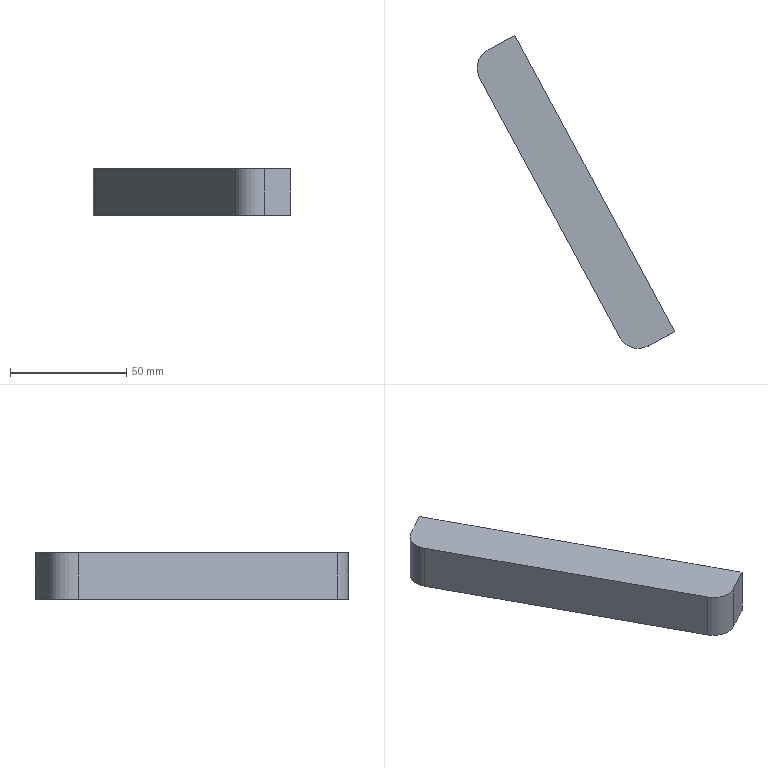Part | Creo | 1 solid | 8 faces | box 85.061 x 134.843 x 20 mm | volume 63105 mm3 | plane 6 | cylinder 2 | commonest cylinder face diameters 18 x2
STEP:
#1=CARTESIAN_POINT('',(0.,0.,0.));
#2=DIRECTION('',(0.,0.,1.));
#3=DIRECTION('',(1.,0.,0.));
#4=AXIS2_PLACEMENT_3D('',#1,#2,#3);
#5=CARTESIAN_POINT('',(223.318,-130.597,-86.844));
#6=VERTEX_POINT('',#5);
#7=CARTESIAN_POINT('',(292.216,-258.183,-86.844));
#8=VERTEX_POINT('',#7);
#9=CARTESIAN_POINT('',(223.318,-130.597,-86.844));
#10=DIRECTION('',(0.4752,-0.8799,0.));
#11=VECTOR('',#10,145.);
#12=LINE('',#9,#11);
#13=EDGE_CURVE('',#6,#8,#12,.T.);
#14=ORIENTED_EDGE('',*,*,#13,.T.);
#15=CARTESIAN_POINT('',(292.216,-258.183,-66.844));
#16=VERTEX_POINT('',#15);
#17=CARTESIAN_POINT('',(292.216,-258.183,-86.844));
#18=DIRECTION('',(0.,0.,1.));
#19=VECTOR('',#18,20.);
#20=LINE('',#17,#19);
#21=EDGE_CURVE('',#8,#16,#20,.T.);
#22=ORIENTED_EDGE('',*,*,#21,.T.);
#23=CARTESIAN_POINT('',(223.318,-130.597,-66.844));
#24=VERTEX_POINT('',#23);
#25=CARTESIAN_POINT('',(292.216,-258.183,-66.844));
#26=DIRECTION('',(-0.4752,0.8799,0.));
#27=VECTOR('',#26,145.);
#28=LINE('',#25,#27);
#29=EDGE_CURVE('',#16,#24,#28,.T.);
#30=ORIENTED_EDGE('',*,*,#29,.T.);
#31=CARTESIAN_POINT('',(223.318,-130.597,-86.844));
#32=DIRECTION('',(0.,0.,1.));
#33=VECTOR('',#32,20.);
#34=LINE('',#31,#33);
#35=EDGE_CURVE('',#6,#24,#34,.T.);
#36=ORIENTED_EDGE('',*,*,#35,.F.);
#37=EDGE_LOOP('',(#14,#22,#30,#36));
#38=FACE_OUTER_BOUND('',#37,.F.);
#39=CARTESIAN_POINT('',(270.834,-218.587,-66.844));
#40=DIRECTION('',(-0.8799,-0.4752,0.));
#41=DIRECTION('',(0.4752,-0.8799,0.));
#42=AXIS2_PLACEMENT_3D('',#39,#40,#41);
#43=PLANE('',#42);
#44=ADVANCED_FACE('',(#38),#43,.F.);
#45=CARTESIAN_POINT('',(280.778,-264.36,-86.844));
#46=VERTEX_POINT('',#45);
#47=CARTESIAN_POINT('',(292.216,-258.183,-86.844));
#48=DIRECTION('',(-0.8799,-0.4752,0.));
#49=VECTOR('',#48,13.);
#50=LINE('',#47,#49);
#51=EDGE_CURVE('',#8,#46,#50,.T.);
#52=ORIENTED_EDGE('',*,*,#51,.F.);
#53=ORIENTED_EDGE('',*,*,#13,.F.);
#54=CARTESIAN_POINT('',(211.879,-136.775,-86.844));
#55=VERTEX_POINT('',#54);
#56=CARTESIAN_POINT('',(211.879,-136.775,-86.844));
#57=DIRECTION('',(0.8799,0.4752,0.));
#58=VECTOR('',#57,13.);
#59=LINE('',#56,#58);
#60=EDGE_CURVE('',#55,#6,#59,.T.);
#61=ORIENTED_EDGE('',*,*,#60,.F.);
#62=CARTESIAN_POINT('',(208.237,-148.97,-86.844));
#63=VERTEX_POINT('',#62);
#64=CARTESIAN_POINT('',(216.156,-144.694,-86.844));
#65=DIRECTION('',(0.,0.,-1.));
#66=DIRECTION('',(-0.8799,-0.4752,0.));
#67=AXIS2_PLACEMENT_3D('',#64,#65,#66);
#68=CIRCLE('',#67,9.);
#69=EDGE_CURVE('',#63,#55,#68,.T.);
#70=ORIENTED_EDGE('',*,*,#69,.F.);
#71=CARTESIAN_POINT('',(268.582,-260.717,-86.844));
#72=VERTEX_POINT('',#71);
#73=CARTESIAN_POINT('',(268.582,-260.717,-86.844));
#74=DIRECTION('',(-0.4752,0.8799,0.));
#75=VECTOR('',#74,127.);
#76=LINE('',#73,#75);
#77=EDGE_CURVE('',#72,#63,#76,.T.);
#78=ORIENTED_EDGE('',*,*,#77,.F.);
#79=CARTESIAN_POINT('',(276.501,-256.441,-86.844));
#80=DIRECTION('',(0.,0.,-1.));
#81=DIRECTION('',(0.4752,-0.8799,0.));
#82=AXIS2_PLACEMENT_3D('',#79,#80,#81);
#83=CIRCLE('',#82,9.);
#84=EDGE_CURVE('',#46,#72,#83,.T.);
#85=ORIENTED_EDGE('',*,*,#84,.F.);
#86=EDGE_LOOP('',(#52,#53,#61,#70,#78,#85));
#87=FACE_OUTER_BOUND('',#86,.F.);
#88=CARTESIAN_POINT('',(270.834,-218.587,-86.844));
#89=DIRECTION('',(0.,0.,-1.));
#90=DIRECTION('',(-1.,0.,0.));
#91=AXIS2_PLACEMENT_3D('',#88,#89,#90);
#92=PLANE('',#91);
#93=ADVANCED_FACE('',(#87),#92,.T.);
#94=CARTESIAN_POINT('',(280.778,-264.36,-66.844));
#95=VERTEX_POINT('',#94);
#96=CARTESIAN_POINT('',(280.778,-264.36,-66.844));
#97=DIRECTION('',(0.8799,0.4752,0.));
#98=VECTOR('',#97,13.);
#99=LINE('',#96,#98);
#100=EDGE_CURVE('',#95,#16,#99,.T.);
#101=ORIENTED_EDGE('',*,*,#100,.T.);
#102=ORIENTED_EDGE('',*,*,#21,.F.);
#103=ORIENTED_EDGE('',*,*,#51,.T.);
#104=CARTESIAN_POINT('',(280.778,-264.36,-86.844));
#105=DIRECTION('',(0.,0.,1.));
#106=VECTOR('',#105,20.);
#107=LINE('',#104,#106);
#108=EDGE_CURVE('',#46,#95,#107,.T.);
#109=ORIENTED_EDGE('',*,*,#108,.T.);
#110=EDGE_LOOP('',(#101,#102,#103,#109));
#111=FACE_OUTER_BOUND('',#110,.F.);
#112=CARTESIAN_POINT('',(292.216,-258.183,-66.844));
#113=DIRECTION('',(0.4752,-0.8799,0.));
#114=DIRECTION('',(0.8799,0.4752,0.));
#115=AXIS2_PLACEMENT_3D('',#112,#113,#114);
#116=PLANE('',#115);
#117=ADVANCED_FACE('',(#111),#116,.T.);
#118=CARTESIAN_POINT('',(208.237,-148.97,-66.844));
#119=VERTEX_POINT('',#118);
#120=CARTESIAN_POINT('',(268.582,-260.717,-66.844));
#121=VERTEX_POINT('',#120);
#122=CARTESIAN_POINT('',(208.237,-148.97,-66.844));
#123=DIRECTION('',(0.4752,-0.8799,0.));
#124=VECTOR('',#123,127.);
#125=LINE('',#122,#124);
#126=EDGE_CURVE('',#119,#121,#125,.T.);
#127=ORIENTED_EDGE('',*,*,#126,.F.);
#128=CARTESIAN_POINT('',(211.879,-136.775,-66.844));
#129=VERTEX_POINT('',#128);
#130=CARTESIAN_POINT('',(216.156,-144.694,-66.844));
#131=DIRECTION('',(0.,0.,1.));
#132=DIRECTION('',(-0.4752,0.8799,0.));
#133=AXIS2_PLACEMENT_3D('',#130,#131,#132);
#134=CIRCLE('',#133,9.);
#135=EDGE_CURVE('',#129,#119,#134,.T.);
#136=ORIENTED_EDGE('',*,*,#135,.F.);
#137=CARTESIAN_POINT('',(223.318,-130.597,-66.844));
#138=DIRECTION('',(-0.8799,-0.4752,0.));
#139=VECTOR('',#138,13.);
#140=LINE('',#137,#139);
#141=EDGE_CURVE('',#24,#129,#140,.T.);
#142=ORIENTED_EDGE('',*,*,#141,.F.);
#143=ORIENTED_EDGE('',*,*,#29,.F.);
#144=ORIENTED_EDGE('',*,*,#100,.F.);
#145=CARTESIAN_POINT('',(276.501,-256.441,-66.844));
#146=DIRECTION('',(0.,0.,1.));
#147=DIRECTION('',(-0.8799,-0.4752,0.));
#148=AXIS2_PLACEMENT_3D('',#145,#146,#147);
#149=CIRCLE('',#148,9.);
#150=EDGE_CURVE('',#121,#95,#149,.T.);
#151=ORIENTED_EDGE('',*,*,#150,.F.);
#152=EDGE_LOOP('',(#127,#136,#142,#143,#144,#151));
#153=FACE_OUTER_BOUND('',#152,.F.);
#154=CARTESIAN_POINT('',(270.834,-218.587,-66.844));
#155=DIRECTION('',(0.,0.,-1.));
#156=DIRECTION('',(-1.,0.,0.));
#157=AXIS2_PLACEMENT_3D('',#154,#155,#156);
#158=PLANE('',#157);
#159=ADVANCED_FACE('',(#153),#158,.F.);
#160=ORIENTED_EDGE('',*,*,#77,.T.);
#161=CARTESIAN_POINT('',(208.237,-148.97,-86.844));
#162=DIRECTION('',(0.,0.,1.));
#163=VECTOR('',#162,20.);
#164=LINE('',#161,#163);
#165=EDGE_CURVE('',#63,#119,#164,.T.);
#166=ORIENTED_EDGE('',*,*,#165,.T.);
#167=ORIENTED_EDGE('',*,*,#126,.T.);
#168=CARTESIAN_POINT('',(268.582,-260.717,-66.844));
#169=DIRECTION('',(0.,0.,-1.));
#170=VECTOR('',#169,20.);
#171=LINE('',#168,#170);
#172=EDGE_CURVE('',#121,#72,#171,.T.);
#173=ORIENTED_EDGE('',*,*,#172,.T.);
#174=EDGE_LOOP('',(#160,#166,#167,#173));
#175=FACE_OUTER_BOUND('',#174,.F.);
#176=CARTESIAN_POINT('',(251.476,-229.041,-66.844));
#177=DIRECTION('',(-0.8799,-0.4752,0.));
#178=DIRECTION('',(0.4752,-0.8799,0.));
#179=AXIS2_PLACEMENT_3D('',#176,#177,#178);
#180=PLANE('',#179);
#181=ADVANCED_FACE('',(#175),#180,.T.);
#182=ORIENTED_EDGE('',*,*,#135,.T.);
#183=ORIENTED_EDGE('',*,*,#165,.F.);
#184=ORIENTED_EDGE('',*,*,#69,.T.);
#185=CARTESIAN_POINT('',(211.879,-136.775,-66.844));
#186=DIRECTION('',(0.,0.,-1.));
#187=VECTOR('',#186,20.);
#188=LINE('',#185,#187);
#189=EDGE_CURVE('',#129,#55,#188,.T.);
#190=ORIENTED_EDGE('',*,*,#189,.F.);
#191=EDGE_LOOP('',(#182,#183,#184,#190));
#192=FACE_OUTER_BOUND('',#191,.F.);
#193=CARTESIAN_POINT('',(216.156,-144.694,-66.844));
#194=DIRECTION('',(0.,0.,-1.));
#195=DIRECTION('',(-1.,0.,0.));
#196=AXIS2_PLACEMENT_3D('',#193,#194,#195);
#197=CYLINDRICAL_SURFACE('',#196,9.);
#198=ADVANCED_FACE('',(#192),#197,.T.);
#199=ORIENTED_EDGE('',*,*,#60,.T.);
#200=ORIENTED_EDGE('',*,*,#35,.T.);
#201=ORIENTED_EDGE('',*,*,#141,.T.);
#202=ORIENTED_EDGE('',*,*,#189,.T.);
#203=EDGE_LOOP('',(#199,#200,#201,#202));
#204=FACE_OUTER_BOUND('',#203,.F.);
#205=CARTESIAN_POINT('',(266.237,-107.421,-29.874));
#206=DIRECTION('',(-0.4752,0.8799,0.));
#207=DIRECTION('',(-0.8799,-0.4752,0.));
#208=AXIS2_PLACEMENT_3D('',#205,#206,#207);
#209=PLANE('',#208);
#210=ADVANCED_FACE('',(#204),#209,.T.);
#211=ORIENTED_EDGE('',*,*,#150,.T.);
#212=ORIENTED_EDGE('',*,*,#108,.F.);
#213=ORIENTED_EDGE('',*,*,#84,.T.);
#214=ORIENTED_EDGE('',*,*,#172,.F.);
#215=EDGE_LOOP('',(#211,#212,#213,#214));
#216=FACE_OUTER_BOUND('',#215,.F.);
#217=CARTESIAN_POINT('',(276.501,-256.441,-66.844));
#218=DIRECTION('',(0.,0.,-1.));
#219=DIRECTION('',(-1.,0.,0.));
#220=AXIS2_PLACEMENT_3D('',#217,#218,#219);
#221=CYLINDRICAL_SURFACE('',#220,9.);
#222=ADVANCED_FACE('',(#216),#221,.T.);
#223=CLOSED_SHELL('',(#44,#93,#117,#159,#181,#198,#210,#222));
#224=MANIFOLD_SOLID_BREP('',#223);
#225=(LENGTH_UNIT()NAMED_UNIT(*)SI_UNIT(.MILLI.,.METRE.));
#226=UNCERTAINTY_MEASURE_WITH_UNIT(LENGTH_MEASURE(0.01607),#225,'','');
#227=(NAMED_UNIT(*)PLANE_ANGLE_UNIT()SI_UNIT($,.RADIAN.));
#228=PLANE_ANGLE_MEASURE_WITH_UNIT(PLANE_ANGLE_MEASURE(0.01745),#227);
#229=(CONVERSION_BASED_UNIT('DEGREE',#228)NAMED_UNIT(*)PLANE_ANGLE_UNIT());
#230=(NAMED_UNIT(*)SI_UNIT($,.STERADIAN.)SOLID_ANGLE_UNIT());
#231=(GEOMETRIC_REPRESENTATION_CONTEXT(3)GLOBAL_UNCERTAINTY_ASSIGNED_CONTEXT((#226))GLOBAL_UNIT_ASSIGNED_CONTEXT((#225,#229,#230))REPRESENTATION_CONTEXT('',''));
#232=ADVANCED_BREP_SHAPE_REPRESENTATION('',(#4,#224),#231);